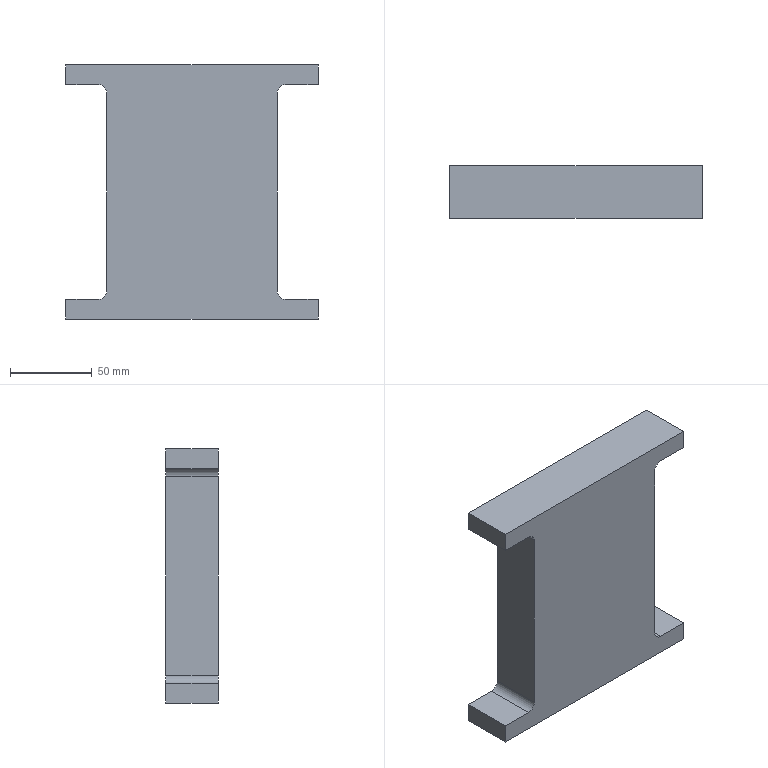Part | NX | 1 solid | 18 faces | box 154 x 32 x 155 mm | volume 554927 mm3 | plane 14 | cylinder 4 | commonest cylinder face diameters 10 x4
STEP:
#1=CARTESIAN_POINT('',(-43.726,-299.015,24.));
#2=VERTEX_POINT('',#1);
#3=CARTESIAN_POINT('',(-63.726,-299.015,24.));
#4=VERTEX_POINT('',#3);
#5=CARTESIAN_POINT('',(-273.242,-299.015,24.));
#6=DIRECTION('',(-1.,0.,0.));
#7=VECTOR('',#6,1000.);
#8=LINE('',#5,#7);
#9=EDGE_CURVE('',#2,#4,#8,.T.);
#10=ORIENTED_EDGE('',*,*,#9,.F.);
#11=CARTESIAN_POINT('',(-38.726,-299.015,29.));
#12=VERTEX_POINT('',#11);
#13=CARTESIAN_POINT('',(-43.726,-299.015,29.));
#14=DIRECTION('',(0.,-1.,0.));
#15=DIRECTION('',(-1.,0.,0.));
#16=AXIS2_PLACEMENT_3D('',#13,#14,#15);
#17=CIRCLE('',#16,5.);
#18=EDGE_CURVE('',#2,#12,#17,.T.);
#19=ORIENTED_EDGE('',*,*,#18,.T.);
#20=CARTESIAN_POINT('',(-38.726,-299.015,150.));
#21=VERTEX_POINT('',#20);
#22=CARTESIAN_POINT('',(-38.726,-299.015,0.));
#23=DIRECTION('',(0.,0.,-1.));
#24=VECTOR('',#23,1000.);
#25=LINE('',#22,#24);
#26=EDGE_CURVE('',#21,#12,#25,.T.);
#27=ORIENTED_EDGE('',*,*,#26,.F.);
#28=CARTESIAN_POINT('',(-43.726,-299.015,155.));
#29=VERTEX_POINT('',#28);
#30=CARTESIAN_POINT('',(-43.726,-299.015,150.));
#31=DIRECTION('',(0.,-1.,0.));
#32=DIRECTION('',(-1.,0.,0.));
#33=AXIS2_PLACEMENT_3D('',#30,#31,#32);
#34=CIRCLE('',#33,5.);
#35=EDGE_CURVE('',#21,#29,#34,.T.);
#36=ORIENTED_EDGE('',*,*,#35,.T.);
#37=CARTESIAN_POINT('',(-63.726,-299.015,155.));
#38=VERTEX_POINT('',#37);
#39=CARTESIAN_POINT('',(-273.242,-299.015,155.));
#40=DIRECTION('',(1.,0.,0.));
#41=VECTOR('',#40,1000.);
#42=LINE('',#39,#41);
#43=EDGE_CURVE('',#38,#29,#42,.T.);
#44=ORIENTED_EDGE('',*,*,#43,.F.);
#45=CARTESIAN_POINT('',(-63.726,-299.015,167.));
#46=VERTEX_POINT('',#45);
#47=CARTESIAN_POINT('',(-63.726,-299.015,0.));
#48=DIRECTION('',(0.,0.,-1.));
#49=VECTOR('',#48,1000.);
#50=LINE('',#47,#49);
#51=EDGE_CURVE('',#46,#38,#50,.T.);
#52=ORIENTED_EDGE('',*,*,#51,.F.);
#53=CARTESIAN_POINT('',(90.274,-299.015,167.));
#54=VERTEX_POINT('',#53);
#55=CARTESIAN_POINT('',(-273.242,-299.015,167.));
#56=DIRECTION('',(-1.,0.,0.));
#57=VECTOR('',#56,1000.);
#58=LINE('',#55,#57);
#59=EDGE_CURVE('',#54,#46,#58,.T.);
#60=ORIENTED_EDGE('',*,*,#59,.F.);
#61=CARTESIAN_POINT('',(90.274,-299.015,155.));
#62=VERTEX_POINT('',#61);
#63=CARTESIAN_POINT('',(90.274,-299.015,0.));
#64=DIRECTION('',(0.,0.,1.));
#65=VECTOR('',#64,1000.);
#66=LINE('',#63,#65);
#67=EDGE_CURVE('',#62,#54,#66,.T.);
#68=ORIENTED_EDGE('',*,*,#67,.F.);
#69=CARTESIAN_POINT('',(70.274,-299.015,155.));
#70=VERTEX_POINT('',#69);
#71=CARTESIAN_POINT('',(-273.242,-299.015,155.));
#72=DIRECTION('',(1.,0.,0.));
#73=VECTOR('',#72,1000.);
#74=LINE('',#71,#73);
#75=EDGE_CURVE('',#70,#62,#74,.T.);
#76=ORIENTED_EDGE('',*,*,#75,.F.);
#77=CARTESIAN_POINT('',(65.274,-299.015,150.));
#78=VERTEX_POINT('',#77);
#79=CARTESIAN_POINT('',(70.274,-299.015,150.));
#80=DIRECTION('',(0.,1.,0.));
#81=DIRECTION('',(1.,0.,0.));
#82=AXIS2_PLACEMENT_3D('',#79,#80,#81);
#83=CIRCLE('',#82,5.);
#84=EDGE_CURVE('',#78,#70,#83,.T.);
#85=ORIENTED_EDGE('',*,*,#84,.F.);
#86=CARTESIAN_POINT('',(65.274,-299.015,29.));
#87=VERTEX_POINT('',#86);
#88=CARTESIAN_POINT('',(65.274,-299.015,0.));
#89=DIRECTION('',(0.,0.,1.));
#90=VECTOR('',#89,1000.);
#91=LINE('',#88,#90);
#92=EDGE_CURVE('',#87,#78,#91,.T.);
#93=ORIENTED_EDGE('',*,*,#92,.F.);
#94=CARTESIAN_POINT('',(70.274,-299.015,24.));
#95=VERTEX_POINT('',#94);
#96=CARTESIAN_POINT('',(70.274,-299.015,29.));
#97=DIRECTION('',(0.,1.,0.));
#98=DIRECTION('',(1.,0.,0.));
#99=AXIS2_PLACEMENT_3D('',#96,#97,#98);
#100=CIRCLE('',#99,5.);
#101=EDGE_CURVE('',#95,#87,#100,.T.);
#102=ORIENTED_EDGE('',*,*,#101,.F.);
#103=CARTESIAN_POINT('',(90.274,-299.015,24.));
#104=VERTEX_POINT('',#103);
#105=CARTESIAN_POINT('',(-273.242,-299.015,24.));
#106=DIRECTION('',(-1.,0.,0.));
#107=VECTOR('',#106,1000.);
#108=LINE('',#105,#107);
#109=EDGE_CURVE('',#104,#95,#108,.T.);
#110=ORIENTED_EDGE('',*,*,#109,.F.);
#111=CARTESIAN_POINT('',(90.274,-299.015,12.));
#112=VERTEX_POINT('',#111);
#113=CARTESIAN_POINT('',(90.274,-299.015,0.));
#114=DIRECTION('',(0.,0.,1.));
#115=VECTOR('',#114,1000.);
#116=LINE('',#113,#115);
#117=EDGE_CURVE('',#112,#104,#116,.T.);
#118=ORIENTED_EDGE('',*,*,#117,.F.);
#119=CARTESIAN_POINT('',(-63.726,-299.015,12.));
#120=VERTEX_POINT('',#119);
#121=CARTESIAN_POINT('',(-273.242,-299.015,12.));
#122=DIRECTION('',(1.,0.,0.));
#123=VECTOR('',#122,1000.);
#124=LINE('',#121,#123);
#125=EDGE_CURVE('',#120,#112,#124,.T.);
#126=ORIENTED_EDGE('',*,*,#125,.F.);
#127=CARTESIAN_POINT('',(-63.726,-299.015,0.));
#128=DIRECTION('',(0.,0.,-1.));
#129=VECTOR('',#128,1000.);
#130=LINE('',#127,#129);
#131=EDGE_CURVE('',#4,#120,#130,.T.);
#132=ORIENTED_EDGE('',*,*,#131,.F.);
#133=EDGE_LOOP('',(#10,#19,#27,#36,#44,#52,#60,#68,#76,#85,#93,#102,#110,#118,#126,#132));
#134=FACE_BOUND('',#133,.T.);
#135=CARTESIAN_POINT('',(119.216,-299.015,309.035));
#136=DIRECTION('',(0.,-1.,0.));
#137=DIRECTION('',(0.,0.,-1.));
#138=AXIS2_PLACEMENT_3D('',#135,#136,#137);
#139=PLANE('',#138);
#140=ADVANCED_FACE('',(#134),#139,.F.);
#141=CARTESIAN_POINT('',(-63.726,-331.015,12.));
#142=VERTEX_POINT('',#141);
#143=CARTESIAN_POINT('',(-63.726,-315.015,12.));
#144=DIRECTION('',(0.,1.,0.));
#145=VECTOR('',#144,1000.);
#146=LINE('',#143,#145);
#147=EDGE_CURVE('',#142,#120,#146,.T.);
#148=ORIENTED_EDGE('',*,*,#147,.F.);
#149=CARTESIAN_POINT('',(-63.726,-331.015,24.));
#150=VERTEX_POINT('',#149);
#151=CARTESIAN_POINT('',(-63.726,-331.015,0.));
#152=DIRECTION('',(0.,0.,-1.));
#153=VECTOR('',#152,1000.);
#154=LINE('',#151,#153);
#155=EDGE_CURVE('',#150,#142,#154,.T.);
#156=ORIENTED_EDGE('',*,*,#155,.F.);
#157=CARTESIAN_POINT('',(-63.726,-315.015,24.));
#158=DIRECTION('',(0.,1.,0.));
#159=VECTOR('',#158,1000.);
#160=LINE('',#157,#159);
#161=EDGE_CURVE('',#150,#4,#160,.T.);
#162=ORIENTED_EDGE('',*,*,#161,.T.);
#163=ORIENTED_EDGE('',*,*,#131,.T.);
#164=EDGE_LOOP('',(#148,#156,#162,#163));
#165=FACE_BOUND('',#164,.T.);
#166=CARTESIAN_POINT('',(-63.726,-315.015,12.));
#167=DIRECTION('',(-1.,0.,0.));
#168=DIRECTION('',(0.,0.,1.));
#169=AXIS2_PLACEMENT_3D('',#166,#167,#168);
#170=PLANE('',#169);
#171=ADVANCED_FACE('',(#165),#170,.T.);
#172=CARTESIAN_POINT('',(-43.726,-331.015,155.));
#173=VERTEX_POINT('',#172);
#174=CARTESIAN_POINT('',(-43.726,-346.647,155.));
#175=DIRECTION('',(0.,-1.,0.));
#176=VECTOR('',#175,1000.);
#177=LINE('',#174,#176);
#178=EDGE_CURVE('',#29,#173,#177,.T.);
#179=ORIENTED_EDGE('',*,*,#178,.T.);
#180=CARTESIAN_POINT('',(-63.726,-331.015,155.));
#181=VERTEX_POINT('',#180);
#182=CARTESIAN_POINT('',(-273.242,-331.015,155.));
#183=DIRECTION('',(1.,0.,0.));
#184=VECTOR('',#183,1000.);
#185=LINE('',#182,#184);
#186=EDGE_CURVE('',#181,#173,#185,.T.);
#187=ORIENTED_EDGE('',*,*,#186,.F.);
#188=CARTESIAN_POINT('',(-63.726,-315.015,155.));
#189=DIRECTION('',(0.,1.,0.));
#190=VECTOR('',#189,1000.);
#191=LINE('',#188,#190);
#192=EDGE_CURVE('',#181,#38,#191,.T.);
#193=ORIENTED_EDGE('',*,*,#192,.T.);
#194=ORIENTED_EDGE('',*,*,#43,.T.);
#195=EDGE_LOOP('',(#179,#187,#193,#194));
#196=FACE_BOUND('',#195,.T.);
#197=CARTESIAN_POINT('',(-63.726,-315.015,155.));
#198=DIRECTION('',(0.,0.,-1.));
#199=DIRECTION('',(0.,-1.,0.));
#200=AXIS2_PLACEMENT_3D('',#197,#198,#199);
#201=PLANE('',#200);
#202=ADVANCED_FACE('',(#196),#201,.T.);
#203=CARTESIAN_POINT('',(90.274,-331.015,24.));
#204=VERTEX_POINT('',#203);
#205=CARTESIAN_POINT('',(90.274,-315.015,24.));
#206=DIRECTION('',(0.,-1.,0.));
#207=VECTOR('',#206,1000.);
#208=LINE('',#205,#207);
#209=EDGE_CURVE('',#104,#204,#208,.T.);
#210=ORIENTED_EDGE('',*,*,#209,.T.);
#211=CARTESIAN_POINT('',(90.274,-331.015,12.));
#212=VERTEX_POINT('',#211);
#213=CARTESIAN_POINT('',(90.274,-331.015,0.));
#214=DIRECTION('',(0.,0.,1.));
#215=VECTOR('',#214,1000.);
#216=LINE('',#213,#215);
#217=EDGE_CURVE('',#212,#204,#216,.T.);
#218=ORIENTED_EDGE('',*,*,#217,.F.);
#219=CARTESIAN_POINT('',(90.274,-315.015,12.));
#220=DIRECTION('',(0.,1.,0.));
#221=VECTOR('',#220,1000.);
#222=LINE('',#219,#221);
#223=EDGE_CURVE('',#212,#112,#222,.T.);
#224=ORIENTED_EDGE('',*,*,#223,.T.);
#225=ORIENTED_EDGE('',*,*,#117,.T.);
#226=EDGE_LOOP('',(#210,#218,#224,#225));
#227=FACE_BOUND('',#226,.T.);
#228=CARTESIAN_POINT('',(90.274,-315.015,24.));
#229=DIRECTION('',(1.,0.,0.));
#230=DIRECTION('',(0.,1.,0.));
#231=AXIS2_PLACEMENT_3D('',#228,#229,#230);
#232=PLANE('',#231);
#233=ADVANCED_FACE('',(#227),#232,.T.);
#234=CARTESIAN_POINT('',(-43.726,-331.015,24.));
#235=VERTEX_POINT('',#234);
#236=CARTESIAN_POINT('',(-43.726,-346.647,24.));
#237=DIRECTION('',(0.,-1.,0.));
#238=VECTOR('',#237,1000.);
#239=LINE('',#236,#238);
#240=EDGE_CURVE('',#2,#235,#239,.T.);
#241=ORIENTED_EDGE('',*,*,#240,.F.);
#242=ORIENTED_EDGE('',*,*,#9,.T.);
#243=ORIENTED_EDGE('',*,*,#161,.F.);
#244=CARTESIAN_POINT('',(-273.242,-331.015,24.));
#245=DIRECTION('',(-1.,0.,0.));
#246=VECTOR('',#245,1000.);
#247=LINE('',#244,#246);
#248=EDGE_CURVE('',#235,#150,#247,.T.);
#249=ORIENTED_EDGE('',*,*,#248,.F.);
#250=EDGE_LOOP('',(#241,#242,#243,#249));
#251=FACE_BOUND('',#250,.T.);
#252=CARTESIAN_POINT('',(-38.726,-315.015,24.));
#253=DIRECTION('',(0.,0.,1.));
#254=DIRECTION('',(1.,0.,0.));
#255=AXIS2_PLACEMENT_3D('',#252,#253,#254);
#256=PLANE('',#255);
#257=ADVANCED_FACE('',(#251),#256,.T.);
#258=CARTESIAN_POINT('',(70.274,-331.015,155.));
#259=VERTEX_POINT('',#258);
#260=CARTESIAN_POINT('',(70.274,-346.647,155.));
#261=DIRECTION('',(0.,1.,0.));
#262=VECTOR('',#261,1000.);
#263=LINE('',#260,#262);
#264=EDGE_CURVE('',#259,#70,#263,.T.);
#265=ORIENTED_EDGE('',*,*,#264,.T.);
#266=ORIENTED_EDGE('',*,*,#75,.T.);
#267=CARTESIAN_POINT('',(90.274,-331.015,155.));
#268=VERTEX_POINT('',#267);
#269=CARTESIAN_POINT('',(90.274,-315.015,155.));
#270=DIRECTION('',(0.,-1.,0.));
#271=VECTOR('',#270,1000.);
#272=LINE('',#269,#271);
#273=EDGE_CURVE('',#62,#268,#272,.T.);
#274=ORIENTED_EDGE('',*,*,#273,.T.);
#275=CARTESIAN_POINT('',(-273.242,-331.015,155.));
#276=DIRECTION('',(1.,0.,0.));
#277=VECTOR('',#276,1000.);
#278=LINE('',#275,#277);
#279=EDGE_CURVE('',#259,#268,#278,.T.);
#280=ORIENTED_EDGE('',*,*,#279,.F.);
#281=EDGE_LOOP('',(#265,#266,#274,#280));
#282=FACE_BOUND('',#281,.T.);
#283=CARTESIAN_POINT('',(65.274,-315.015,155.));
#284=DIRECTION('',(0.,0.,-1.));
#285=DIRECTION('',(0.,-1.,0.));
#286=AXIS2_PLACEMENT_3D('',#283,#284,#285);
#287=PLANE('',#286);
#288=ADVANCED_FACE('',(#282),#287,.T.);
#289=ORIENTED_EDGE('',*,*,#273,.F.);
#290=ORIENTED_EDGE('',*,*,#67,.T.);
#291=CARTESIAN_POINT('',(90.274,-331.015,167.));
#292=VERTEX_POINT('',#291);
#293=CARTESIAN_POINT('',(90.274,-315.015,167.));
#294=DIRECTION('',(0.,-1.,0.));
#295=VECTOR('',#294,1000.);
#296=LINE('',#293,#295);
#297=EDGE_CURVE('',#54,#292,#296,.T.);
#298=ORIENTED_EDGE('',*,*,#297,.T.);
#299=CARTESIAN_POINT('',(90.274,-331.015,0.));
#300=DIRECTION('',(0.,0.,1.));
#301=VECTOR('',#300,1000.);
#302=LINE('',#299,#301);
#303=EDGE_CURVE('',#268,#292,#302,.T.);
#304=ORIENTED_EDGE('',*,*,#303,.F.);
#305=EDGE_LOOP('',(#289,#290,#298,#304));
#306=FACE_BOUND('',#305,.T.);
#307=CARTESIAN_POINT('',(90.274,-315.015,155.));
#308=DIRECTION('',(1.,0.,0.));
#309=DIRECTION('',(0.,1.,0.));
#310=AXIS2_PLACEMENT_3D('',#307,#308,#309);
#311=PLANE('',#310);
#312=ADVANCED_FACE('',(#306),#311,.T.);
#313=CARTESIAN_POINT('',(65.274,-331.015,150.));
#314=VERTEX_POINT('',#313);
#315=CARTESIAN_POINT('',(65.274,-346.647,150.));
#316=DIRECTION('',(0.,1.,0.));
#317=VECTOR('',#316,1000.);
#318=LINE('',#315,#317);
#319=EDGE_CURVE('',#314,#78,#318,.T.);
#320=ORIENTED_EDGE('',*,*,#319,.F.);
#321=CARTESIAN_POINT('',(65.274,-331.015,29.));
#322=VERTEX_POINT('',#321);
#323=CARTESIAN_POINT('',(65.274,-331.015,0.));
#324=DIRECTION('',(0.,0.,1.));
#325=VECTOR('',#324,1000.);
#326=LINE('',#323,#325);
#327=EDGE_CURVE('',#322,#314,#326,.T.);
#328=ORIENTED_EDGE('',*,*,#327,.F.);
#329=CARTESIAN_POINT('',(65.274,-346.647,29.));
#330=DIRECTION('',(0.,1.,0.));
#331=VECTOR('',#330,1000.);
#332=LINE('',#329,#331);
#333=EDGE_CURVE('',#322,#87,#332,.T.);
#334=ORIENTED_EDGE('',*,*,#333,.T.);
#335=ORIENTED_EDGE('',*,*,#92,.T.);
#336=EDGE_LOOP('',(#320,#328,#334,#335));
#337=FACE_BOUND('',#336,.T.);
#338=CARTESIAN_POINT('',(65.274,-315.015,24.));
#339=DIRECTION('',(1.,0.,0.));
#340=DIRECTION('',(0.,1.,0.));
#341=AXIS2_PLACEMENT_3D('',#338,#339,#340);
#342=PLANE('',#341);
#343=ADVANCED_FACE('',(#337),#342,.T.);
#344=CARTESIAN_POINT('',(-63.726,-331.015,167.));
#345=VERTEX_POINT('',#344);
#346=CARTESIAN_POINT('',(-63.726,-315.015,167.));
#347=DIRECTION('',(0.,-1.,0.));
#348=VECTOR('',#347,1000.);
#349=LINE('',#346,#348);
#350=EDGE_CURVE('',#46,#345,#349,.T.);
#351=ORIENTED_EDGE('',*,*,#350,.T.);
#352=CARTESIAN_POINT('',(-273.242,-331.015,167.));
#353=DIRECTION('',(-1.,0.,0.));
#354=VECTOR('',#353,1000.);
#355=LINE('',#352,#354);
#356=EDGE_CURVE('',#292,#345,#355,.T.);
#357=ORIENTED_EDGE('',*,*,#356,.F.);
#358=ORIENTED_EDGE('',*,*,#297,.F.);
#359=ORIENTED_EDGE('',*,*,#59,.T.);
#360=EDGE_LOOP('',(#351,#357,#358,#359));
#361=FACE_BOUND('',#360,.T.);
#362=CARTESIAN_POINT('',(-63.726,-315.015,167.));
#363=DIRECTION('',(0.,0.,1.));
#364=DIRECTION('',(1.,0.,0.));
#365=AXIS2_PLACEMENT_3D('',#362,#363,#364);
#366=PLANE('',#365);
#367=ADVANCED_FACE('',(#361),#366,.T.);
#368=ORIENTED_EDGE('',*,*,#192,.F.);
#369=CARTESIAN_POINT('',(-63.726,-331.015,0.));
#370=DIRECTION('',(0.,0.,-1.));
#371=VECTOR('',#370,1000.);
#372=LINE('',#369,#371);
#373=EDGE_CURVE('',#345,#181,#372,.T.);
#374=ORIENTED_EDGE('',*,*,#373,.F.);
#375=ORIENTED_EDGE('',*,*,#350,.F.);
#376=ORIENTED_EDGE('',*,*,#51,.T.);
#377=EDGE_LOOP('',(#368,#374,#375,#376));
#378=FACE_BOUND('',#377,.T.);
#379=CARTESIAN_POINT('',(-63.726,-315.015,155.));
#380=DIRECTION('',(-1.,0.,0.));
#381=DIRECTION('',(0.,0.,1.));
#382=AXIS2_PLACEMENT_3D('',#379,#380,#381);
#383=PLANE('',#382);
#384=ADVANCED_FACE('',(#378),#383,.T.);
#385=ORIENTED_EDGE('',*,*,#209,.F.);
#386=ORIENTED_EDGE('',*,*,#109,.T.);
#387=CARTESIAN_POINT('',(70.274,-331.015,24.));
#388=VERTEX_POINT('',#387);
#389=CARTESIAN_POINT('',(70.274,-346.647,24.));
#390=DIRECTION('',(0.,1.,0.));
#391=VECTOR('',#390,1000.);
#392=LINE('',#389,#391);
#393=EDGE_CURVE('',#388,#95,#392,.T.);
#394=ORIENTED_EDGE('',*,*,#393,.F.);
#395=CARTESIAN_POINT('',(-273.242,-331.015,24.));
#396=DIRECTION('',(-1.,0.,0.));
#397=VECTOR('',#396,1000.);
#398=LINE('',#395,#397);
#399=EDGE_CURVE('',#204,#388,#398,.T.);
#400=ORIENTED_EDGE('',*,*,#399,.F.);
#401=EDGE_LOOP('',(#385,#386,#394,#400));
#402=FACE_BOUND('',#401,.T.);
#403=CARTESIAN_POINT('',(90.274,-315.015,24.));
#404=DIRECTION('',(0.,0.,1.));
#405=DIRECTION('',(1.,0.,0.));
#406=AXIS2_PLACEMENT_3D('',#403,#404,#405);
#407=PLANE('',#406);
#408=ADVANCED_FACE('',(#402),#407,.T.);
#409=CARTESIAN_POINT('',(-38.726,-331.015,29.));
#410=VERTEX_POINT('',#409);
#411=CARTESIAN_POINT('',(-38.726,-346.647,29.));
#412=DIRECTION('',(0.,-1.,0.));
#413=VECTOR('',#412,1000.);
#414=LINE('',#411,#413);
#415=EDGE_CURVE('',#12,#410,#414,.T.);
#416=ORIENTED_EDGE('',*,*,#415,.T.);
#417=CARTESIAN_POINT('',(-38.726,-331.015,150.));
#418=VERTEX_POINT('',#417);
#419=CARTESIAN_POINT('',(-38.726,-331.015,0.));
#420=DIRECTION('',(0.,0.,-1.));
#421=VECTOR('',#420,1000.);
#422=LINE('',#419,#421);
#423=EDGE_CURVE('',#418,#410,#422,.T.);
#424=ORIENTED_EDGE('',*,*,#423,.F.);
#425=CARTESIAN_POINT('',(-38.726,-346.647,150.));
#426=DIRECTION('',(0.,-1.,0.));
#427=VECTOR('',#426,1000.);
#428=LINE('',#425,#427);
#429=EDGE_CURVE('',#21,#418,#428,.T.);
#430=ORIENTED_EDGE('',*,*,#429,.F.);
#431=ORIENTED_EDGE('',*,*,#26,.T.);
#432=EDGE_LOOP('',(#416,#424,#430,#431));
#433=FACE_BOUND('',#432,.T.);
#434=CARTESIAN_POINT('',(-38.726,-315.015,24.));
#435=DIRECTION('',(-1.,0.,0.));
#436=DIRECTION('',(0.,0.,1.));
#437=AXIS2_PLACEMENT_3D('',#434,#435,#436);
#438=PLANE('',#437);
#439=ADVANCED_FACE('',(#433),#438,.T.);
#440=ORIENTED_EDGE('',*,*,#178,.F.);
#441=ORIENTED_EDGE('',*,*,#35,.F.);
#442=ORIENTED_EDGE('',*,*,#429,.T.);
#443=CARTESIAN_POINT('',(-43.726,-331.015,150.));
#444=DIRECTION('',(0.,-1.,0.));
#445=DIRECTION('',(-1.,0.,0.));
#446=AXIS2_PLACEMENT_3D('',#443,#444,#445);
#447=CIRCLE('',#446,5.);
#448=EDGE_CURVE('',#418,#173,#447,.T.);
#449=ORIENTED_EDGE('',*,*,#448,.T.);
#450=EDGE_LOOP('',(#440,#441,#442,#449));
#451=FACE_BOUND('',#450,.T.);
#452=CARTESIAN_POINT('',(-43.726,-346.647,150.));
#453=DIRECTION('',(0.,-1.,0.));
#454=DIRECTION('',(-1.,0.,0.));
#455=AXIS2_PLACEMENT_3D('',#452,#453,#454);
#456=CYLINDRICAL_SURFACE('',#455,5.);
#457=ADVANCED_FACE('',(#451),#456,.F.);
#458=ORIENTED_EDGE('',*,*,#240,.T.);
#459=CARTESIAN_POINT('',(-43.726,-331.015,29.));
#460=DIRECTION('',(0.,-1.,0.));
#461=DIRECTION('',(-1.,0.,0.));
#462=AXIS2_PLACEMENT_3D('',#459,#460,#461);
#463=CIRCLE('',#462,5.);
#464=EDGE_CURVE('',#235,#410,#463,.T.);
#465=ORIENTED_EDGE('',*,*,#464,.T.);
#466=ORIENTED_EDGE('',*,*,#415,.F.);
#467=ORIENTED_EDGE('',*,*,#18,.F.);
#468=EDGE_LOOP('',(#458,#465,#466,#467));
#469=FACE_BOUND('',#468,.T.);
#470=CARTESIAN_POINT('',(-43.726,-346.647,29.));
#471=DIRECTION('',(0.,-1.,0.));
#472=DIRECTION('',(-1.,0.,0.));
#473=AXIS2_PLACEMENT_3D('',#470,#471,#472);
#474=CYLINDRICAL_SURFACE('',#473,5.);
#475=ADVANCED_FACE('',(#469),#474,.F.);
#476=ORIENTED_EDGE('',*,*,#333,.F.);
#477=CARTESIAN_POINT('',(70.274,-331.015,29.));
#478=DIRECTION('',(0.,1.,0.));
#479=DIRECTION('',(1.,0.,0.));
#480=AXIS2_PLACEMENT_3D('',#477,#478,#479);
#481=CIRCLE('',#480,5.);
#482=EDGE_CURVE('',#388,#322,#481,.T.);
#483=ORIENTED_EDGE('',*,*,#482,.F.);
#484=ORIENTED_EDGE('',*,*,#393,.T.);
#485=ORIENTED_EDGE('',*,*,#101,.T.);
#486=EDGE_LOOP('',(#476,#483,#484,#485));
#487=FACE_BOUND('',#486,.T.);
#488=CARTESIAN_POINT('',(70.274,-346.647,29.));
#489=DIRECTION('',(0.,1.,0.));
#490=DIRECTION('',(1.,0.,0.));
#491=AXIS2_PLACEMENT_3D('',#488,#489,#490);
#492=CYLINDRICAL_SURFACE('',#491,5.);
#493=ADVANCED_FACE('',(#487),#492,.F.);
#494=ORIENTED_EDGE('',*,*,#319,.T.);
#495=ORIENTED_EDGE('',*,*,#84,.T.);
#496=ORIENTED_EDGE('',*,*,#264,.F.);
#497=CARTESIAN_POINT('',(70.274,-331.015,150.));
#498=DIRECTION('',(0.,1.,0.));
#499=DIRECTION('',(1.,0.,0.));
#500=AXIS2_PLACEMENT_3D('',#497,#498,#499);
#501=CIRCLE('',#500,5.);
#502=EDGE_CURVE('',#314,#259,#501,.T.);
#503=ORIENTED_EDGE('',*,*,#502,.F.);
#504=EDGE_LOOP('',(#494,#495,#496,#503));
#505=FACE_BOUND('',#504,.T.);
#506=CARTESIAN_POINT('',(70.274,-346.647,150.));
#507=DIRECTION('',(0.,1.,0.));
#508=DIRECTION('',(1.,0.,0.));
#509=AXIS2_PLACEMENT_3D('',#506,#507,#508);
#510=CYLINDRICAL_SURFACE('',#509,5.);
#511=ADVANCED_FACE('',(#505),#510,.F.);
#512=ORIENTED_EDGE('',*,*,#155,.T.);
#513=CARTESIAN_POINT('',(-273.242,-331.015,12.));
#514=DIRECTION('',(1.,0.,0.));
#515=VECTOR('',#514,1000.);
#516=LINE('',#513,#515);
#517=EDGE_CURVE('',#142,#212,#516,.T.);
#518=ORIENTED_EDGE('',*,*,#517,.T.);
#519=ORIENTED_EDGE('',*,*,#217,.T.);
#520=ORIENTED_EDGE('',*,*,#399,.T.);
#521=ORIENTED_EDGE('',*,*,#482,.T.);
#522=ORIENTED_EDGE('',*,*,#327,.T.);
#523=ORIENTED_EDGE('',*,*,#502,.T.);
#524=ORIENTED_EDGE('',*,*,#279,.T.);
#525=ORIENTED_EDGE('',*,*,#303,.T.);
#526=ORIENTED_EDGE('',*,*,#356,.T.);
#527=ORIENTED_EDGE('',*,*,#373,.T.);
#528=ORIENTED_EDGE('',*,*,#186,.T.);
#529=ORIENTED_EDGE('',*,*,#448,.F.);
#530=ORIENTED_EDGE('',*,*,#423,.T.);
#531=ORIENTED_EDGE('',*,*,#464,.F.);
#532=ORIENTED_EDGE('',*,*,#248,.T.);
#533=EDGE_LOOP('',(#512,#518,#519,#520,#521,#522,#523,#524,#525,#526,#527,#528,#529,#530,#531,#532));
#534=FACE_BOUND('',#533,.T.);
#535=CARTESIAN_POINT('',(119.216,-331.015,309.035));
#536=DIRECTION('',(0.,-1.,0.));
#537=DIRECTION('',(0.,0.,-1.));
#538=AXIS2_PLACEMENT_3D('',#535,#536,#537);
#539=PLANE('',#538);
#540=ADVANCED_FACE('',(#534),#539,.T.);
#541=ORIENTED_EDGE('',*,*,#147,.T.);
#542=ORIENTED_EDGE('',*,*,#125,.T.);
#543=ORIENTED_EDGE('',*,*,#223,.F.);
#544=ORIENTED_EDGE('',*,*,#517,.F.);
#545=EDGE_LOOP('',(#541,#542,#543,#544));
#546=FACE_BOUND('',#545,.T.);
#547=CARTESIAN_POINT('',(-63.726,-315.015,12.));
#548=DIRECTION('',(0.,0.,-1.));
#549=DIRECTION('',(0.,-1.,0.));
#550=AXIS2_PLACEMENT_3D('',#547,#548,#549);
#551=PLANE('',#550);
#552=ADVANCED_FACE('',(#546),#551,.T.);
#553=CLOSED_SHELL('',(#140,#171,#202,#233,#257,#288,#312,#343,#367,#384,#408,#439,#457,#475,#493,#511,#540,#552));
#554=MANIFOLD_SOLID_BREP('',#553);
#555=(LENGTH_UNIT()NAMED_UNIT(*)SI_UNIT(.MILLI.,.METRE.));
#556=UNCERTAINTY_MEASURE_WITH_UNIT(LENGTH_MEASURE(0.00001),#555,'','');
#557=(NAMED_UNIT(*)PLANE_ANGLE_UNIT()SI_UNIT($,.RADIAN.));
#558=(NAMED_UNIT(*)SI_UNIT($,.STERADIAN.)SOLID_ANGLE_UNIT());
#559=(GEOMETRIC_REPRESENTATION_CONTEXT(3)GLOBAL_UNCERTAINTY_ASSIGNED_CONTEXT((#556))GLOBAL_UNIT_ASSIGNED_CONTEXT((#555,#557,#558))REPRESENTATION_CONTEXT('',''));
#560=ADVANCED_BREP_SHAPE_REPRESENTATION('',(#554),#559);